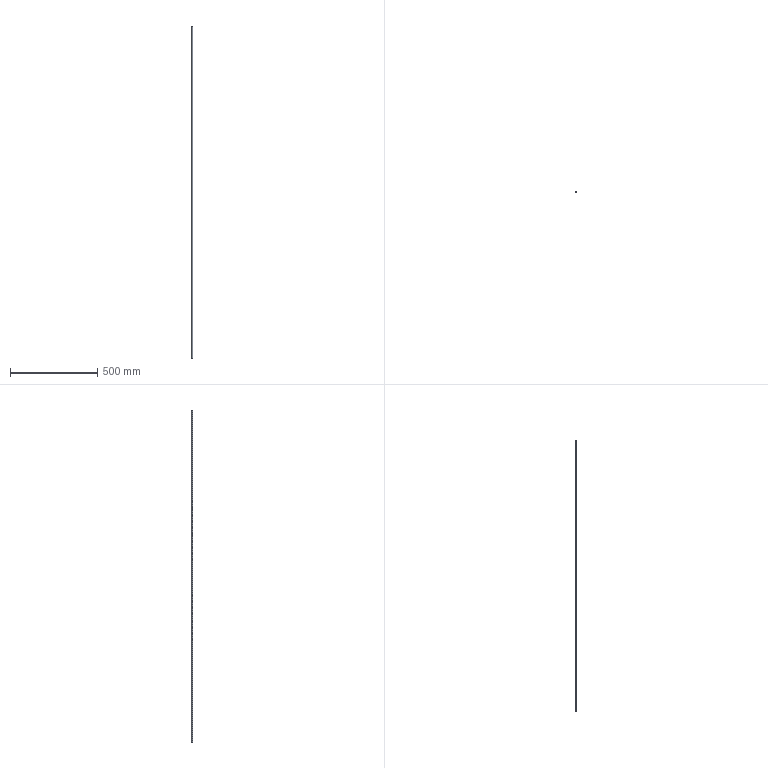Part | SolidWorks | features Extrusion 1 | 1 solid | 6 faces | box 6 x 6 x 1900 mm | volume 23503 mm3 | cylinder 4 | plane 2 | commonest cylinder face diameters 4.5 x2 6 x2
STEP:
#1=CARTESIAN_POINT('',(-2.25,0.,1900.));
#2=VERTEX_POINT('',#1);
#3=CARTESIAN_POINT('',(2.25,0.,1900.));
#4=VERTEX_POINT('',#3);
#5=CARTESIAN_POINT('',(0.,0.,1900.));
#6=DIRECTION('',(0.,0.,1.));
#7=DIRECTION('',(1.,0.,0.));
#8=AXIS2_PLACEMENT_3D('',#5,#6,#7);
#9=CIRCLE('',#8,2.25);
#10=EDGE_CURVE('',#2,#4,#9,.T.);
#11=ORIENTED_EDGE('',*,*,#10,.T.);
#12=CARTESIAN_POINT('',(2.25,0.,0.));
#13=VERTEX_POINT('',#12);
#14=CARTESIAN_POINT('',(2.25,0.,1900.));
#15=DIRECTION('',(0.,0.,-1.));
#16=VECTOR('',#15,1000.);
#17=LINE('',#14,#16);
#18=EDGE_CURVE('',#4,#13,#17,.T.);
#19=ORIENTED_EDGE('',*,*,#18,.T.);
#20=CARTESIAN_POINT('',(-2.25,0.,0.));
#21=VERTEX_POINT('',#20);
#22=CARTESIAN_POINT('',(0.,0.,0.));
#23=DIRECTION('',(0.,0.,1.));
#24=DIRECTION('',(1.,0.,0.));
#25=AXIS2_PLACEMENT_3D('',#22,#23,#24);
#26=CIRCLE('',#25,2.25);
#27=EDGE_CURVE('',#21,#13,#26,.T.);
#28=ORIENTED_EDGE('',*,*,#27,.F.);
#29=CARTESIAN_POINT('',(-2.25,0.,1900.));
#30=DIRECTION('',(0.,0.,-1.));
#31=VECTOR('',#30,1000.);
#32=LINE('',#29,#31);
#33=EDGE_CURVE('',#2,#21,#32,.T.);
#34=ORIENTED_EDGE('',*,*,#33,.F.);
#35=EDGE_LOOP('',(#11,#19,#28,#34));
#36=FACE_OUTER_BOUND('',#35,.T.);
#37=CARTESIAN_POINT('',(0.,0.,1900.));
#38=DIRECTION('',(0.,0.,-1.));
#39=DIRECTION('',(-1.,0.,0.));
#40=AXIS2_PLACEMENT_3D('',#37,#38,#39);
#41=CYLINDRICAL_SURFACE('',#40,2.25);
#42=ADVANCED_FACE('',(#36),#41,.F.);
#43=CARTESIAN_POINT('',(3.,0.,1900.));
#44=VERTEX_POINT('',#43);
#45=CARTESIAN_POINT('',(-3.,0.,1900.));
#46=VERTEX_POINT('',#45);
#47=CARTESIAN_POINT('',(0.,0.,1900.));
#48=DIRECTION('',(0.,0.,1.));
#49=DIRECTION('',(1.,0.,0.));
#50=AXIS2_PLACEMENT_3D('',#47,#48,#49);
#51=CIRCLE('',#50,3.);
#52=EDGE_CURVE('',#44,#46,#51,.T.);
#53=ORIENTED_EDGE('',*,*,#52,.F.);
#54=CARTESIAN_POINT('',(3.,0.,0.));
#55=VERTEX_POINT('',#54);
#56=CARTESIAN_POINT('',(3.,0.,1900.));
#57=DIRECTION('',(0.,0.,-1.));
#58=VECTOR('',#57,1000.);
#59=LINE('',#56,#58);
#60=EDGE_CURVE('',#44,#55,#59,.T.);
#61=ORIENTED_EDGE('',*,*,#60,.T.);
#62=CARTESIAN_POINT('',(-3.,0.,0.));
#63=VERTEX_POINT('',#62);
#64=CARTESIAN_POINT('',(0.,0.,0.));
#65=DIRECTION('',(0.,0.,1.));
#66=DIRECTION('',(1.,0.,0.));
#67=AXIS2_PLACEMENT_3D('',#64,#65,#66);
#68=CIRCLE('',#67,3.);
#69=EDGE_CURVE('',#55,#63,#68,.T.);
#70=ORIENTED_EDGE('',*,*,#69,.T.);
#71=CARTESIAN_POINT('',(-3.,0.,1900.));
#72=DIRECTION('',(0.,0.,-1.));
#73=VECTOR('',#72,1000.);
#74=LINE('',#71,#73);
#75=EDGE_CURVE('',#46,#63,#74,.T.);
#76=ORIENTED_EDGE('',*,*,#75,.F.);
#77=EDGE_LOOP('',(#53,#61,#70,#76));
#78=FACE_OUTER_BOUND('',#77,.T.);
#79=CARTESIAN_POINT('',(0.,0.,1900.));
#80=DIRECTION('',(0.,0.,-1.));
#81=DIRECTION('',(-1.,0.,0.));
#82=AXIS2_PLACEMENT_3D('',#79,#80,#81);
#83=CYLINDRICAL_SURFACE('',#82,3.);
#84=ADVANCED_FACE('',(#78),#83,.T.);
#85=CARTESIAN_POINT('',(0.,0.,1900.));
#86=DIRECTION('',(0.,0.,1.));
#87=DIRECTION('',(1.,0.,0.));
#88=AXIS2_PLACEMENT_3D('',#85,#86,#87);
#89=CIRCLE('',#88,3.);
#90=EDGE_CURVE('',#46,#44,#89,.T.);
#91=ORIENTED_EDGE('',*,*,#90,.T.);
#92=ORIENTED_EDGE('',*,*,#52,.T.);
#93=EDGE_LOOP('',(#91,#92));
#94=FACE_OUTER_BOUND('',#93,.T.);
#95=ORIENTED_EDGE('',*,*,#10,.F.);
#96=CARTESIAN_POINT('',(0.,0.,1900.));
#97=DIRECTION('',(0.,0.,1.));
#98=DIRECTION('',(1.,0.,0.));
#99=AXIS2_PLACEMENT_3D('',#96,#97,#98);
#100=CIRCLE('',#99,2.25);
#101=EDGE_CURVE('',#4,#2,#100,.T.);
#102=ORIENTED_EDGE('',*,*,#101,.F.);
#103=EDGE_LOOP('',(#95,#102));
#104=FACE_BOUND('',#103,.T.);
#105=CARTESIAN_POINT('',(0.,0.,1900.));
#106=DIRECTION('',(0.,0.,1.));
#107=DIRECTION('',(1.,0.,0.));
#108=AXIS2_PLACEMENT_3D('',#105,#106,#107);
#109=PLANE('',#108);
#110=ADVANCED_FACE('',(#94,#104),#109,.T.);
#111=CARTESIAN_POINT('',(0.,0.,0.));
#112=DIRECTION('',(0.,0.,1.));
#113=DIRECTION('',(1.,0.,0.));
#114=AXIS2_PLACEMENT_3D('',#111,#112,#113);
#115=CIRCLE('',#114,3.);
#116=EDGE_CURVE('',#63,#55,#115,.T.);
#117=ORIENTED_EDGE('',*,*,#116,.F.);
#118=ORIENTED_EDGE('',*,*,#69,.F.);
#119=EDGE_LOOP('',(#117,#118));
#120=FACE_OUTER_BOUND('',#119,.T.);
#121=ORIENTED_EDGE('',*,*,#27,.T.);
#122=CARTESIAN_POINT('',(0.,0.,0.));
#123=DIRECTION('',(0.,0.,1.));
#124=DIRECTION('',(1.,0.,0.));
#125=AXIS2_PLACEMENT_3D('',#122,#123,#124);
#126=CIRCLE('',#125,2.25);
#127=EDGE_CURVE('',#13,#21,#126,.T.);
#128=ORIENTED_EDGE('',*,*,#127,.T.);
#129=EDGE_LOOP('',(#121,#128));
#130=FACE_BOUND('',#129,.T.);
#131=CARTESIAN_POINT('',(0.,0.,0.));
#132=DIRECTION('',(0.,0.,1.));
#133=DIRECTION('',(1.,0.,0.));
#134=AXIS2_PLACEMENT_3D('',#131,#132,#133);
#135=PLANE('',#134);
#136=ADVANCED_FACE('',(#120,#130),#135,.F.);
#137=ORIENTED_EDGE('',*,*,#60,.F.);
#138=ORIENTED_EDGE('',*,*,#90,.F.);
#139=ORIENTED_EDGE('',*,*,#75,.T.);
#140=ORIENTED_EDGE('',*,*,#116,.T.);
#141=EDGE_LOOP('',(#137,#138,#139,#140));
#142=FACE_OUTER_BOUND('',#141,.T.);
#143=CARTESIAN_POINT('',(0.,0.,1900.));
#144=DIRECTION('',(0.,0.,-1.));
#145=DIRECTION('',(-1.,0.,0.));
#146=AXIS2_PLACEMENT_3D('',#143,#144,#145);
#147=CYLINDRICAL_SURFACE('',#146,3.);
#148=ADVANCED_FACE('',(#142),#147,.T.);
#149=ORIENTED_EDGE('',*,*,#18,.F.);
#150=ORIENTED_EDGE('',*,*,#101,.T.);
#151=ORIENTED_EDGE('',*,*,#33,.T.);
#152=ORIENTED_EDGE('',*,*,#127,.F.);
#153=EDGE_LOOP('',(#149,#150,#151,#152));
#154=FACE_OUTER_BOUND('',#153,.T.);
#155=CARTESIAN_POINT('',(0.,0.,1900.));
#156=DIRECTION('',(0.,0.,-1.));
#157=DIRECTION('',(-1.,0.,0.));
#158=AXIS2_PLACEMENT_3D('',#155,#156,#157);
#159=CYLINDRICAL_SURFACE('',#158,2.25);
#160=ADVANCED_FACE('',(#154),#159,.F.);
#161=CLOSED_SHELL('',(#42,#84,#110,#136,#148,#160));
#162=MANIFOLD_SOLID_BREP('',#161);
#163=CARTESIAN_POINT('',(0.,0.,0.));
#164=DIRECTION('',(0.,0.,1.));
#165=DIRECTION('',(1.,0.,0.));
#166=AXIS2_PLACEMENT_3D('',#163,#164,#165);
#167=(LENGTH_UNIT()NAMED_UNIT(*)SI_UNIT(.MILLI.,.METRE.));
#168=UNCERTAINTY_MEASURE_WITH_UNIT(LENGTH_MEASURE(0.00001),#167,'','');
#169=(NAMED_UNIT(*)PLANE_ANGLE_UNIT()SI_UNIT($,.RADIAN.));
#170=(NAMED_UNIT(*)SI_UNIT($,.STERADIAN.)SOLID_ANGLE_UNIT());
#171=(GEOMETRIC_REPRESENTATION_CONTEXT(3)GLOBAL_UNCERTAINTY_ASSIGNED_CONTEXT((#168))GLOBAL_UNIT_ASSIGNED_CONTEXT((#167,#169,#170))REPRESENTATION_CONTEXT('',''));
#172=ADVANCED_BREP_SHAPE_REPRESENTATION('',(#162,#166),#171);